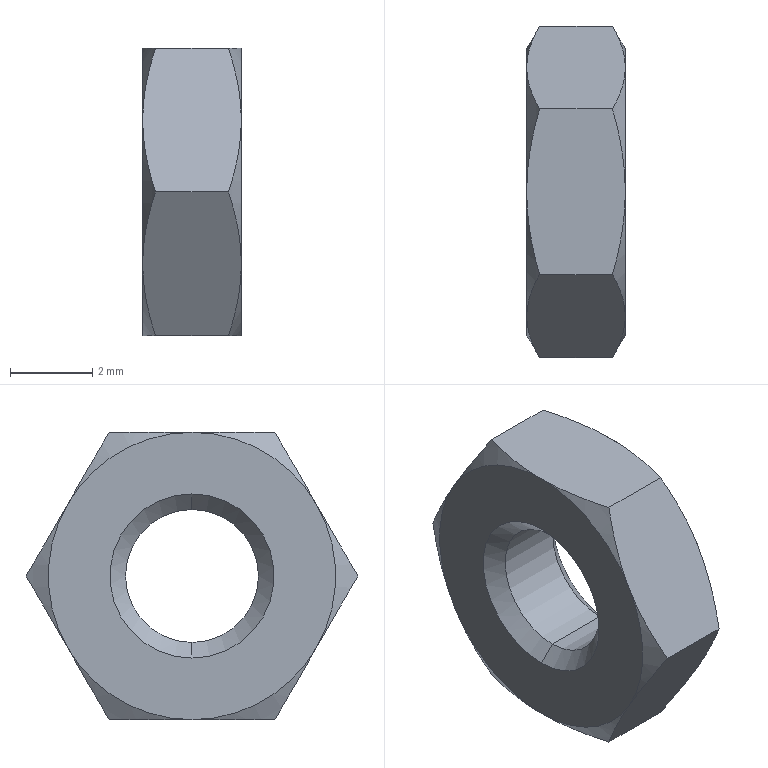Part | STEP file | 0246_Z_002_PUST4-25_2 | 1 solid | 26 faces | box 2.4 x 8.083 x 7 mm | volume 79.701 mm3 | cone 16 | plane 8 | cylinder 2 | commonest cylinder face diameters 3.242 x2